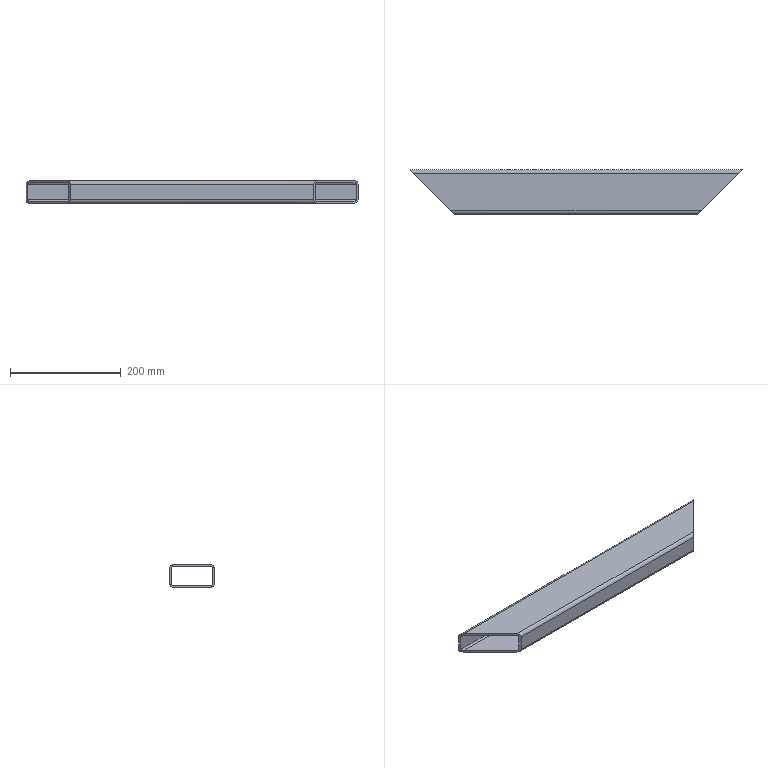Part | SolidWorks | features 3DProfileFeature 1, ICE 1, WeldMemberFeat 1, WeldmentFeature 1 | 1 solid | 18 faces | box 600 x 80 x 40 mm | volume 343628 mm3 | plane 10 | cylinder 8 | commonest cylinder face diameters 6 x4 12 x4
STEP:
#1=CARTESIAN_POINT('',(526.,-34.,-20.));
#2=VERTEX_POINT('',#1);
#3=CARTESIAN_POINT('',(594.,34.,-20.));
#4=VERTEX_POINT('',#3);
#5=CARTESIAN_POINT('',(280.,-280.,-20.));
#6=DIRECTION('',(0.7071,0.7071,0.));
#7=VECTOR('',#6,1000.);
#8=LINE('',#5,#7);
#9=EDGE_CURVE('',#2,#4,#8,.T.);
#10=ORIENTED_EDGE('',*,*,#9,.F.);
#11=CARTESIAN_POINT('',(74.,-34.,-20.));
#12=VERTEX_POINT('',#11);
#13=CARTESIAN_POINT('',(600.,-34.,-20.));
#14=DIRECTION('',(-1.,0.,0.));
#15=VECTOR('',#14,1000.);
#16=LINE('',#13,#15);
#17=EDGE_CURVE('',#2,#12,#16,.T.);
#18=ORIENTED_EDGE('',*,*,#17,.T.);
#19=CARTESIAN_POINT('',(6.,34.,-20.));
#20=VERTEX_POINT('',#19);
#21=CARTESIAN_POINT('',(20.,20.,-20.));
#22=DIRECTION('',(0.7071,-0.7071,0.));
#23=VECTOR('',#22,1000.);
#24=LINE('',#21,#23);
#25=EDGE_CURVE('',#20,#12,#24,.T.);
#26=ORIENTED_EDGE('',*,*,#25,.F.);
#27=CARTESIAN_POINT('',(600.,34.,-20.));
#28=DIRECTION('',(-1.,0.,0.));
#29=VECTOR('',#28,1000.);
#30=LINE('',#27,#29);
#31=EDGE_CURVE('',#4,#20,#30,.T.);
#32=ORIENTED_EDGE('',*,*,#31,.F.);
#33=EDGE_LOOP('',(#10,#18,#26,#32));
#34=FACE_OUTER_BOUND('',#33,.T.);
#35=CARTESIAN_POINT('',(600.,34.,-20.));
#36=DIRECTION('',(0.,0.,1.));
#37=DIRECTION('',(1.,0.,0.));
#38=AXIS2_PLACEMENT_3D('',#35,#36,#37);
#39=PLANE('',#38);
#40=ADVANCED_FACE('',(#34),#39,.F.);
#41=CARTESIAN_POINT('',(520.,-40.,-14.));
#42=VERTEX_POINT('',#41);
#43=CARTESIAN_POINT('',(520.,-40.,-14.));
#44=CARTESIAN_POINT('',(520.,-40.,-17.515));
#45=CARTESIAN_POINT('',(522.485,-37.515,-20.));
#46=CARTESIAN_POINT('',(526.,-34.,-20.));
#47=(BOUNDED_CURVE()B_SPLINE_CURVE(3,(#43,#44,#45,#46),.UNSPECIFIED.,.F.,.F.)B_SPLINE_CURVE_WITH_KNOTS((4,4),(0.,1.571),.UNSPECIFIED.)CURVE()GEOMETRIC_REPRESENTATION_ITEM()RATIONAL_B_SPLINE_CURVE((1.,0.8047,0.8047,1.))REPRESENTATION_ITEM(''));
#48=EDGE_CURVE('',#42,#2,#47,.T.);
#49=ORIENTED_EDGE('',*,*,#48,.F.);
#50=CARTESIAN_POINT('',(80.,-40.,-14.));
#51=VERTEX_POINT('',#50);
#52=CARTESIAN_POINT('',(600.,-40.,-14.));
#53=DIRECTION('',(-1.,0.,0.));
#54=VECTOR('',#53,1000.);
#55=LINE('',#52,#54);
#56=EDGE_CURVE('',#42,#51,#55,.T.);
#57=ORIENTED_EDGE('',*,*,#56,.T.);
#58=CARTESIAN_POINT('',(74.,-34.,-20.));
#59=CARTESIAN_POINT('',(77.515,-37.515,-20.));
#60=CARTESIAN_POINT('',(80.,-40.,-17.515));
#61=CARTESIAN_POINT('',(80.,-40.,-14.));
#62=(BOUNDED_CURVE()B_SPLINE_CURVE(3,(#58,#59,#60,#61),.UNSPECIFIED.,.F.,.F.)B_SPLINE_CURVE_WITH_KNOTS((4,4),(1.571,3.142),.UNSPECIFIED.)CURVE()GEOMETRIC_REPRESENTATION_ITEM()RATIONAL_B_SPLINE_CURVE((1.,0.8047,0.8047,1.))REPRESENTATION_ITEM(''));
#63=EDGE_CURVE('',#12,#51,#62,.T.);
#64=ORIENTED_EDGE('',*,*,#63,.F.);
#65=ORIENTED_EDGE('',*,*,#17,.F.);
#66=EDGE_LOOP('',(#49,#57,#64,#65));
#67=FACE_OUTER_BOUND('',#66,.T.);
#68=CARTESIAN_POINT('',(600.,-34.,-14.));
#69=DIRECTION('',(-1.,0.,0.));
#70=DIRECTION('',(0.,0.,1.));
#71=AXIS2_PLACEMENT_3D('',#68,#69,#70);
#72=CYLINDRICAL_SURFACE('',#71,6.);
#73=ADVANCED_FACE('',(#67),#72,.T.);
#74=CARTESIAN_POINT('',(520.,-40.,14.));
#75=VERTEX_POINT('',#74);
#76=CARTESIAN_POINT('',(520.,-40.,-20.));
#77=DIRECTION('',(0.,0.,1.));
#78=VECTOR('',#77,1000.);
#79=LINE('',#76,#78);
#80=EDGE_CURVE('',#42,#75,#79,.T.);
#81=ORIENTED_EDGE('',*,*,#80,.T.);
#82=CARTESIAN_POINT('',(80.,-40.,14.));
#83=VERTEX_POINT('',#82);
#84=CARTESIAN_POINT('',(600.,-40.,14.));
#85=DIRECTION('',(-1.,0.,0.));
#86=VECTOR('',#85,1000.);
#87=LINE('',#84,#86);
#88=EDGE_CURVE('',#75,#83,#87,.T.);
#89=ORIENTED_EDGE('',*,*,#88,.T.);
#90=CARTESIAN_POINT('',(80.,-40.,-20.));
#91=DIRECTION('',(0.,0.,1.));
#92=VECTOR('',#91,1000.);
#93=LINE('',#90,#92);
#94=EDGE_CURVE('',#51,#83,#93,.T.);
#95=ORIENTED_EDGE('',*,*,#94,.F.);
#96=ORIENTED_EDGE('',*,*,#56,.F.);
#97=EDGE_LOOP('',(#81,#89,#95,#96));
#98=FACE_OUTER_BOUND('',#97,.T.);
#99=CARTESIAN_POINT('',(600.,-40.,14.));
#100=DIRECTION('',(0.,1.,0.));
#101=DIRECTION('',(0.,0.,1.));
#102=AXIS2_PLACEMENT_3D('',#99,#100,#101);
#103=PLANE('',#102);
#104=ADVANCED_FACE('',(#98),#103,.F.);
#105=CARTESIAN_POINT('',(526.,-34.,20.));
#106=VERTEX_POINT('',#105);
#107=CARTESIAN_POINT('',(526.,-34.,20.));
#108=CARTESIAN_POINT('',(522.485,-37.515,20.));
#109=CARTESIAN_POINT('',(520.,-40.,17.515));
#110=CARTESIAN_POINT('',(520.,-40.,14.));
#111=(BOUNDED_CURVE()B_SPLINE_CURVE(3,(#107,#108,#109,#110),.UNSPECIFIED.,.F.,.F.)B_SPLINE_CURVE_WITH_KNOTS((4,4),(4.712,6.283),.UNSPECIFIED.)CURVE()GEOMETRIC_REPRESENTATION_ITEM()RATIONAL_B_SPLINE_CURVE((1.,0.8047,0.8047,1.))REPRESENTATION_ITEM(''));
#112=EDGE_CURVE('',#106,#75,#111,.T.);
#113=ORIENTED_EDGE('',*,*,#112,.F.);
#114=CARTESIAN_POINT('',(74.,-34.,20.));
#115=VERTEX_POINT('',#114);
#116=CARTESIAN_POINT('',(600.,-34.,20.));
#117=DIRECTION('',(-1.,0.,0.));
#118=VECTOR('',#117,1000.);
#119=LINE('',#116,#118);
#120=EDGE_CURVE('',#106,#115,#119,.T.);
#121=ORIENTED_EDGE('',*,*,#120,.T.);
#122=CARTESIAN_POINT('',(80.,-40.,14.));
#123=CARTESIAN_POINT('',(80.,-40.,17.515));
#124=CARTESIAN_POINT('',(77.515,-37.515,20.));
#125=CARTESIAN_POINT('',(74.,-34.,20.));
#126=(BOUNDED_CURVE()B_SPLINE_CURVE(3,(#122,#123,#124,#125),.UNSPECIFIED.,.F.,.F.)B_SPLINE_CURVE_WITH_KNOTS((4,4),(3.142,4.712),.UNSPECIFIED.)CURVE()GEOMETRIC_REPRESENTATION_ITEM()RATIONAL_B_SPLINE_CURVE((1.,0.8047,0.8047,1.))REPRESENTATION_ITEM(''));
#127=EDGE_CURVE('',#83,#115,#126,.T.);
#128=ORIENTED_EDGE('',*,*,#127,.F.);
#129=ORIENTED_EDGE('',*,*,#88,.F.);
#130=EDGE_LOOP('',(#113,#121,#128,#129));
#131=FACE_OUTER_BOUND('',#130,.T.);
#132=CARTESIAN_POINT('',(600.,-34.,14.));
#133=DIRECTION('',(-1.,0.,0.));
#134=DIRECTION('',(0.,0.,1.));
#135=AXIS2_PLACEMENT_3D('',#132,#133,#134);
#136=CYLINDRICAL_SURFACE('',#135,6.);
#137=ADVANCED_FACE('',(#131),#136,.T.);
#138=CARTESIAN_POINT('',(594.,34.,20.));
#139=VERTEX_POINT('',#138);
#140=CARTESIAN_POINT('',(280.,-280.,20.));
#141=DIRECTION('',(0.7071,0.7071,0.));
#142=VECTOR('',#141,1000.);
#143=LINE('',#140,#142);
#144=EDGE_CURVE('',#106,#139,#143,.T.);
#145=ORIENTED_EDGE('',*,*,#144,.T.);
#146=CARTESIAN_POINT('',(6.,34.,20.));
#147=VERTEX_POINT('',#146);
#148=CARTESIAN_POINT('',(600.,34.,20.));
#149=DIRECTION('',(-1.,0.,0.));
#150=VECTOR('',#149,1000.);
#151=LINE('',#148,#150);
#152=EDGE_CURVE('',#139,#147,#151,.T.);
#153=ORIENTED_EDGE('',*,*,#152,.T.);
#154=CARTESIAN_POINT('',(20.,20.,20.));
#155=DIRECTION('',(0.7071,-0.7071,0.));
#156=VECTOR('',#155,1000.);
#157=LINE('',#154,#156);
#158=EDGE_CURVE('',#147,#115,#157,.T.);
#159=ORIENTED_EDGE('',*,*,#158,.T.);
#160=ORIENTED_EDGE('',*,*,#120,.F.);
#161=EDGE_LOOP('',(#145,#153,#159,#160));
#162=FACE_OUTER_BOUND('',#161,.T.);
#163=CARTESIAN_POINT('',(600.,-34.,20.));
#164=DIRECTION('',(0.,0.,-1.));
#165=DIRECTION('',(-1.,0.,0.));
#166=AXIS2_PLACEMENT_3D('',#163,#164,#165);
#167=PLANE('',#166);
#168=ADVANCED_FACE('',(#162),#167,.F.);
#169=CARTESIAN_POINT('',(0.,40.,-14.));
#170=VERTEX_POINT('',#169);
#171=CARTESIAN_POINT('',(0.,40.,14.));
#172=VERTEX_POINT('',#171);
#173=CARTESIAN_POINT('',(0.,40.,-14.));
#174=DIRECTION('',(0.,0.,1.));
#175=VECTOR('',#174,1000.);
#176=LINE('',#173,#175);
#177=EDGE_CURVE('',#170,#172,#176,.T.);
#178=ORIENTED_EDGE('',*,*,#177,.T.);
#179=CARTESIAN_POINT('',(600.,40.,14.));
#180=VERTEX_POINT('',#179);
#181=CARTESIAN_POINT('',(600.,40.,14.));
#182=DIRECTION('',(-1.,0.,0.));
#183=VECTOR('',#182,1000.);
#184=LINE('',#181,#183);
#185=EDGE_CURVE('',#180,#172,#184,.T.);
#186=ORIENTED_EDGE('',*,*,#185,.F.);
#187=CARTESIAN_POINT('',(600.,40.,-14.));
#188=VERTEX_POINT('',#187);
#189=CARTESIAN_POINT('',(600.,40.,-14.));
#190=DIRECTION('',(0.,0.,1.));
#191=VECTOR('',#190,1000.);
#192=LINE('',#189,#191);
#193=EDGE_CURVE('',#188,#180,#192,.T.);
#194=ORIENTED_EDGE('',*,*,#193,.F.);
#195=CARTESIAN_POINT('',(600.,40.,-14.));
#196=DIRECTION('',(-1.,0.,0.));
#197=VECTOR('',#196,1000.);
#198=LINE('',#195,#197);
#199=EDGE_CURVE('',#188,#170,#198,.T.);
#200=ORIENTED_EDGE('',*,*,#199,.T.);
#201=EDGE_LOOP('',(#178,#186,#194,#200));
#202=FACE_OUTER_BOUND('',#201,.T.);
#203=CARTESIAN_POINT('',(600.,40.,-14.));
#204=DIRECTION('',(0.,-1.,0.));
#205=DIRECTION('',(0.,0.,-1.));
#206=AXIS2_PLACEMENT_3D('',#203,#204,#205);
#207=PLANE('',#206);
#208=ADVANCED_FACE('',(#202),#207,.F.);
#209=CARTESIAN_POINT('',(600.,40.,14.));
#210=CARTESIAN_POINT('',(600.,40.,17.515));
#211=CARTESIAN_POINT('',(597.515,37.515,20.));
#212=CARTESIAN_POINT('',(594.,34.,20.));
#213=(BOUNDED_CURVE()B_SPLINE_CURVE(3,(#209,#210,#211,#212),.UNSPECIFIED.,.F.,.F.)B_SPLINE_CURVE_WITH_KNOTS((4,4),(3.142,4.712),.UNSPECIFIED.)CURVE()GEOMETRIC_REPRESENTATION_ITEM()RATIONAL_B_SPLINE_CURVE((1.,0.8047,0.8047,1.))REPRESENTATION_ITEM(''));
#214=EDGE_CURVE('',#180,#139,#213,.T.);
#215=ORIENTED_EDGE('',*,*,#214,.F.);
#216=ORIENTED_EDGE('',*,*,#185,.T.);
#217=CARTESIAN_POINT('',(6.,34.,20.));
#218=CARTESIAN_POINT('',(2.485,37.515,20.));
#219=CARTESIAN_POINT('',(0.,40.,17.515));
#220=CARTESIAN_POINT('',(0.,40.,14.));
#221=(BOUNDED_CURVE()B_SPLINE_CURVE(3,(#217,#218,#219,#220),.UNSPECIFIED.,.F.,.F.)B_SPLINE_CURVE_WITH_KNOTS((4,4),(4.712,6.283),.UNSPECIFIED.)CURVE()GEOMETRIC_REPRESENTATION_ITEM()RATIONAL_B_SPLINE_CURVE((1.,0.8047,0.8047,1.))REPRESENTATION_ITEM(''));
#222=EDGE_CURVE('',#147,#172,#221,.T.);
#223=ORIENTED_EDGE('',*,*,#222,.F.);
#224=ORIENTED_EDGE('',*,*,#152,.F.);
#225=EDGE_LOOP('',(#215,#216,#223,#224));
#226=FACE_OUTER_BOUND('',#225,.T.);
#227=CARTESIAN_POINT('',(600.,34.,14.));
#228=DIRECTION('',(-1.,0.,0.));
#229=DIRECTION('',(0.,0.,1.));
#230=AXIS2_PLACEMENT_3D('',#227,#228,#229);
#231=CYLINDRICAL_SURFACE('',#230,6.);
#232=ADVANCED_FACE('',(#226),#231,.T.);
#233=CARTESIAN_POINT('',(594.,34.,-20.));
#234=CARTESIAN_POINT('',(597.515,37.515,-20.));
#235=CARTESIAN_POINT('',(600.,40.,-17.515));
#236=CARTESIAN_POINT('',(600.,40.,-14.));
#237=(BOUNDED_CURVE()B_SPLINE_CURVE(3,(#233,#234,#235,#236),.UNSPECIFIED.,.F.,.F.)B_SPLINE_CURVE_WITH_KNOTS((4,4),(1.571,3.142),.UNSPECIFIED.)CURVE()GEOMETRIC_REPRESENTATION_ITEM()RATIONAL_B_SPLINE_CURVE((1.,0.8047,0.8047,1.))REPRESENTATION_ITEM(''));
#238=EDGE_CURVE('',#4,#188,#237,.T.);
#239=ORIENTED_EDGE('',*,*,#238,.F.);
#240=ORIENTED_EDGE('',*,*,#31,.T.);
#241=CARTESIAN_POINT('',(0.,40.,-14.));
#242=CARTESIAN_POINT('',(0.,40.,-17.515));
#243=CARTESIAN_POINT('',(2.485,37.515,-20.));
#244=CARTESIAN_POINT('',(6.,34.,-20.));
#245=(BOUNDED_CURVE()B_SPLINE_CURVE(3,(#241,#242,#243,#244),.UNSPECIFIED.,.F.,.F.)B_SPLINE_CURVE_WITH_KNOTS((4,4),(0.,1.571),.UNSPECIFIED.)CURVE()GEOMETRIC_REPRESENTATION_ITEM()RATIONAL_B_SPLINE_CURVE((1.,0.8047,0.8047,1.))REPRESENTATION_ITEM(''));
#246=EDGE_CURVE('',#170,#20,#245,.T.);
#247=ORIENTED_EDGE('',*,*,#246,.F.);
#248=ORIENTED_EDGE('',*,*,#199,.F.);
#249=EDGE_LOOP('',(#239,#240,#247,#248));
#250=FACE_OUTER_BOUND('',#249,.T.);
#251=CARTESIAN_POINT('',(600.,34.,-14.));
#252=DIRECTION('',(-1.,0.,0.));
#253=DIRECTION('',(0.,0.,1.));
#254=AXIS2_PLACEMENT_3D('',#251,#252,#253);
#255=CYLINDRICAL_SURFACE('',#254,6.);
#256=ADVANCED_FACE('',(#250),#255,.T.);
#257=CARTESIAN_POINT('',(74.,-34.,17.));
#258=VERTEX_POINT('',#257);
#259=CARTESIAN_POINT('',(6.,34.,17.));
#260=VERTEX_POINT('',#259);
#261=CARTESIAN_POINT('',(337.,-297.,17.));
#262=DIRECTION('',(-0.7071,0.7071,0.));
#263=VECTOR('',#262,1000.);
#264=LINE('',#261,#263);
#265=EDGE_CURVE('',#258,#260,#264,.T.);
#266=ORIENTED_EDGE('',*,*,#265,.F.);
#267=CARTESIAN_POINT('',(77.,-37.,14.));
#268=VERTEX_POINT('',#267);
#269=CARTESIAN_POINT('',(77.,-37.,14.));
#270=CARTESIAN_POINT('',(77.,-37.,15.757));
#271=CARTESIAN_POINT('',(75.757,-35.757,17.));
#272=CARTESIAN_POINT('',(74.,-34.,17.));
#273=(BOUNDED_CURVE()B_SPLINE_CURVE(3,(#269,#270,#271,#272),.UNSPECIFIED.,.F.,.T.)B_SPLINE_CURVE_WITH_KNOTS((4,4),(3.142,4.712),.UNSPECIFIED.)CURVE()GEOMETRIC_REPRESENTATION_ITEM()RATIONAL_B_SPLINE_CURVE((1.,0.8047,0.8047,1.))REPRESENTATION_ITEM(''));
#274=EDGE_CURVE('',#268,#258,#273,.T.);
#275=ORIENTED_EDGE('',*,*,#274,.F.);
#276=CARTESIAN_POINT('',(77.,-37.,-14.));
#277=VERTEX_POINT('',#276);
#278=CARTESIAN_POINT('',(77.,-37.,14.));
#279=DIRECTION('',(0.,0.,1.));
#280=VECTOR('',#279,1000.);
#281=LINE('',#278,#280);
#282=EDGE_CURVE('',#277,#268,#281,.T.);
#283=ORIENTED_EDGE('',*,*,#282,.F.);
#284=CARTESIAN_POINT('',(74.,-34.,-17.));
#285=VERTEX_POINT('',#284);
#286=CARTESIAN_POINT('',(74.,-34.,-17.));
#287=CARTESIAN_POINT('',(75.757,-35.757,-17.));
#288=CARTESIAN_POINT('',(77.,-37.,-15.757));
#289=CARTESIAN_POINT('',(77.,-37.,-14.));
#290=(BOUNDED_CURVE()B_SPLINE_CURVE(3,(#286,#287,#288,#289),.UNSPECIFIED.,.F.,.F.)B_SPLINE_CURVE_WITH_KNOTS((4,4),(1.571,3.142),.UNSPECIFIED.)CURVE()GEOMETRIC_REPRESENTATION_ITEM()RATIONAL_B_SPLINE_CURVE((1.,0.8047,0.8047,1.))REPRESENTATION_ITEM(''));
#291=EDGE_CURVE('',#285,#277,#290,.T.);
#292=ORIENTED_EDGE('',*,*,#291,.F.);
#293=CARTESIAN_POINT('',(6.,34.,-17.));
#294=VERTEX_POINT('',#293);
#295=CARTESIAN_POINT('',(303.,-263.,-17.));
#296=DIRECTION('',(0.7071,-0.7071,0.));
#297=VECTOR('',#296,1000.);
#298=LINE('',#295,#297);
#299=EDGE_CURVE('',#294,#285,#298,.T.);
#300=ORIENTED_EDGE('',*,*,#299,.F.);
#301=CARTESIAN_POINT('',(3.,37.,-14.));
#302=VERTEX_POINT('',#301);
#303=CARTESIAN_POINT('',(3.,37.,-14.));
#304=CARTESIAN_POINT('',(3.,37.,-15.757));
#305=CARTESIAN_POINT('',(4.243,35.757,-17.));
#306=CARTESIAN_POINT('',(6.,34.,-17.));
#307=(BOUNDED_CURVE()B_SPLINE_CURVE(3,(#303,#304,#305,#306),.UNSPECIFIED.,.F.,.F.)B_SPLINE_CURVE_WITH_KNOTS((4,4),(0.,1.571),.UNSPECIFIED.)CURVE()GEOMETRIC_REPRESENTATION_ITEM()RATIONAL_B_SPLINE_CURVE((1.,0.8047,0.8047,1.))REPRESENTATION_ITEM(''));
#308=EDGE_CURVE('',#302,#294,#307,.T.);
#309=ORIENTED_EDGE('',*,*,#308,.F.);
#310=CARTESIAN_POINT('',(3.,37.,14.));
#311=VERTEX_POINT('',#310);
#312=CARTESIAN_POINT('',(3.,37.,-14.));
#313=DIRECTION('',(0.,0.,-1.));
#314=VECTOR('',#313,1000.);
#315=LINE('',#312,#314);
#316=EDGE_CURVE('',#311,#302,#315,.T.);
#317=ORIENTED_EDGE('',*,*,#316,.F.);
#318=CARTESIAN_POINT('',(6.,34.,17.));
#319=CARTESIAN_POINT('',(4.243,35.757,17.));
#320=CARTESIAN_POINT('',(3.,37.,15.757));
#321=CARTESIAN_POINT('',(3.,37.,14.));
#322=(BOUNDED_CURVE()B_SPLINE_CURVE(3,(#318,#319,#320,#321),.UNSPECIFIED.,.F.,.F.)B_SPLINE_CURVE_WITH_KNOTS((4,4),(4.712,6.283),.UNSPECIFIED.)CURVE()GEOMETRIC_REPRESENTATION_ITEM()RATIONAL_B_SPLINE_CURVE((1.,0.8047,0.8047,1.))REPRESENTATION_ITEM(''));
#323=EDGE_CURVE('',#260,#311,#322,.T.);
#324=ORIENTED_EDGE('',*,*,#323,.F.);
#325=EDGE_LOOP('',(#266,#275,#283,#292,#300,#309,#317,#324));
#326=FACE_BOUND('',#325,.T.);
#327=ORIENTED_EDGE('',*,*,#246,.T.);
#328=ORIENTED_EDGE('',*,*,#25,.T.);
#329=ORIENTED_EDGE('',*,*,#63,.T.);
#330=ORIENTED_EDGE('',*,*,#94,.T.);
#331=ORIENTED_EDGE('',*,*,#127,.T.);
#332=ORIENTED_EDGE('',*,*,#158,.F.);
#333=ORIENTED_EDGE('',*,*,#222,.T.);
#334=ORIENTED_EDGE('',*,*,#177,.F.);
#335=EDGE_LOOP('',(#327,#328,#329,#330,#331,#332,#333,#334));
#336=FACE_OUTER_BOUND('',#335,.T.);
#337=CARTESIAN_POINT('',(20.,20.,-20.));
#338=DIRECTION('',(-0.7071,-0.7071,0.));
#339=DIRECTION('',(0.7071,-0.7071,0.));
#340=AXIS2_PLACEMENT_3D('',#337,#338,#339);
#341=PLANE('',#340);
#342=ADVANCED_FACE('',(#326,#336),#341,.T.);
#343=CARTESIAN_POINT('',(597.,37.,-14.));
#344=VERTEX_POINT('',#343);
#345=CARTESIAN_POINT('',(597.,37.,14.));
#346=VERTEX_POINT('',#345);
#347=CARTESIAN_POINT('',(597.,37.,-14.));
#348=DIRECTION('',(0.,0.,1.));
#349=VECTOR('',#348,1000.);
#350=LINE('',#347,#349);
#351=EDGE_CURVE('',#344,#346,#350,.T.);
#352=ORIENTED_EDGE('',*,*,#351,.F.);
#353=CARTESIAN_POINT('',(594.,34.,-17.));
#354=VERTEX_POINT('',#353);
#355=CARTESIAN_POINT('',(594.,34.,-17.));
#356=CARTESIAN_POINT('',(595.757,35.757,-17.));
#357=CARTESIAN_POINT('',(597.,37.,-15.757));
#358=CARTESIAN_POINT('',(597.,37.,-14.));
#359=(BOUNDED_CURVE()B_SPLINE_CURVE(3,(#355,#356,#357,#358),.UNSPECIFIED.,.F.,.F.)B_SPLINE_CURVE_WITH_KNOTS((4,4),(1.571,3.142),.UNSPECIFIED.)CURVE()GEOMETRIC_REPRESENTATION_ITEM()RATIONAL_B_SPLINE_CURVE((1.,0.8047,0.8047,1.))REPRESENTATION_ITEM(''));
#360=EDGE_CURVE('',#354,#344,#359,.T.);
#361=ORIENTED_EDGE('',*,*,#360,.F.);
#362=CARTESIAN_POINT('',(526.,-34.,-17.));
#363=VERTEX_POINT('',#362);
#364=CARTESIAN_POINT('',(597.,37.,-17.));
#365=DIRECTION('',(0.7071,0.7071,0.));
#366=VECTOR('',#365,1000.);
#367=LINE('',#364,#366);
#368=EDGE_CURVE('',#363,#354,#367,.T.);
#369=ORIENTED_EDGE('',*,*,#368,.F.);
#370=CARTESIAN_POINT('',(523.,-37.,-14.));
#371=VERTEX_POINT('',#370);
#372=CARTESIAN_POINT('',(523.,-37.,-14.));
#373=CARTESIAN_POINT('',(523.,-37.,-15.757));
#374=CARTESIAN_POINT('',(524.243,-35.757,-17.));
#375=CARTESIAN_POINT('',(526.,-34.,-17.));
#376=(BOUNDED_CURVE()B_SPLINE_CURVE(3,(#372,#373,#374,#375),.UNSPECIFIED.,.F.,.F.)B_SPLINE_CURVE_WITH_KNOTS((4,4),(0.,1.571),.UNSPECIFIED.)CURVE()GEOMETRIC_REPRESENTATION_ITEM()RATIONAL_B_SPLINE_CURVE((1.,0.8047,0.8047,1.))REPRESENTATION_ITEM(''));
#377=EDGE_CURVE('',#371,#363,#376,.T.);
#378=ORIENTED_EDGE('',*,*,#377,.F.);
#379=CARTESIAN_POINT('',(523.,-37.,14.));
#380=VERTEX_POINT('',#379);
#381=CARTESIAN_POINT('',(523.,-37.,14.));
#382=DIRECTION('',(0.,0.,-1.));
#383=VECTOR('',#382,1000.);
#384=LINE('',#381,#383);
#385=EDGE_CURVE('',#380,#371,#384,.T.);
#386=ORIENTED_EDGE('',*,*,#385,.F.);
#387=CARTESIAN_POINT('',(526.,-34.,17.));
#388=VERTEX_POINT('',#387);
#389=CARTESIAN_POINT('',(526.,-34.,17.));
#390=CARTESIAN_POINT('',(524.243,-35.757,17.));
#391=CARTESIAN_POINT('',(523.,-37.,15.757));
#392=CARTESIAN_POINT('',(523.,-37.,14.));
#393=(BOUNDED_CURVE()B_SPLINE_CURVE(3,(#389,#390,#391,#392),.UNSPECIFIED.,.F.,.F.)B_SPLINE_CURVE_WITH_KNOTS((4,4),(4.712,6.283),.UNSPECIFIED.)CURVE()GEOMETRIC_REPRESENTATION_ITEM()RATIONAL_B_SPLINE_CURVE((1.,0.8047,0.8047,1.))REPRESENTATION_ITEM(''));
#394=EDGE_CURVE('',#388,#380,#393,.T.);
#395=ORIENTED_EDGE('',*,*,#394,.F.);
#396=CARTESIAN_POINT('',(594.,34.,17.));
#397=VERTEX_POINT('',#396);
#398=CARTESIAN_POINT('',(563.,3.,17.));
#399=DIRECTION('',(-0.7071,-0.7071,0.));
#400=VECTOR('',#399,1000.);
#401=LINE('',#398,#400);
#402=EDGE_CURVE('',#397,#388,#401,.T.);
#403=ORIENTED_EDGE('',*,*,#402,.F.);
#404=CARTESIAN_POINT('',(597.,37.,14.));
#405=CARTESIAN_POINT('',(597.,37.,15.757));
#406=CARTESIAN_POINT('',(595.757,35.757,17.));
#407=CARTESIAN_POINT('',(594.,34.,17.));
#408=(BOUNDED_CURVE()B_SPLINE_CURVE(3,(#404,#405,#406,#407),.UNSPECIFIED.,.F.,.F.)B_SPLINE_CURVE_WITH_KNOTS((4,4),(3.142,4.712),.UNSPECIFIED.)CURVE()GEOMETRIC_REPRESENTATION_ITEM()RATIONAL_B_SPLINE_CURVE((1.,0.8047,0.8047,1.))REPRESENTATION_ITEM(''));
#409=EDGE_CURVE('',#346,#397,#408,.T.);
#410=ORIENTED_EDGE('',*,*,#409,.F.);
#411=EDGE_LOOP('',(#352,#361,#369,#378,#386,#395,#403,#410));
#412=FACE_BOUND('',#411,.T.);
#413=ORIENTED_EDGE('',*,*,#238,.T.);
#414=ORIENTED_EDGE('',*,*,#193,.T.);
#415=ORIENTED_EDGE('',*,*,#214,.T.);
#416=ORIENTED_EDGE('',*,*,#144,.F.);
#417=ORIENTED_EDGE('',*,*,#112,.T.);
#418=ORIENTED_EDGE('',*,*,#80,.F.);
#419=ORIENTED_EDGE('',*,*,#48,.T.);
#420=ORIENTED_EDGE('',*,*,#9,.T.);
#421=EDGE_LOOP('',(#413,#414,#415,#416,#417,#418,#419,#420));
#422=FACE_OUTER_BOUND('',#421,.T.);
#423=CARTESIAN_POINT('',(280.,-280.,-20.));
#424=DIRECTION('',(0.7071,-0.7071,0.));
#425=DIRECTION('',(0.7071,0.7071,0.));
#426=AXIS2_PLACEMENT_3D('',#423,#424,#425);
#427=PLANE('',#426);
#428=ADVANCED_FACE('',(#412,#422),#427,.T.);
#429=CARTESIAN_POINT('',(600.,37.,14.));
#430=DIRECTION('',(-1.,0.,0.));
#431=VECTOR('',#430,1000.);
#432=LINE('',#429,#431);
#433=EDGE_CURVE('',#346,#311,#432,.T.);
#434=ORIENTED_EDGE('',*,*,#433,.F.);
#435=ORIENTED_EDGE('',*,*,#409,.T.);
#436=CARTESIAN_POINT('',(600.,34.,17.));
#437=DIRECTION('',(-1.,0.,0.));
#438=VECTOR('',#437,1000.);
#439=LINE('',#436,#438);
#440=EDGE_CURVE('',#397,#260,#439,.T.);
#441=ORIENTED_EDGE('',*,*,#440,.T.);
#442=ORIENTED_EDGE('',*,*,#323,.T.);
#443=EDGE_LOOP('',(#434,#435,#441,#442));
#444=FACE_OUTER_BOUND('',#443,.T.);
#445=CARTESIAN_POINT('',(600.,34.,14.));
#446=DIRECTION('',(-1.,0.,0.));
#447=DIRECTION('',(0.,0.,1.));
#448=AXIS2_PLACEMENT_3D('',#445,#446,#447);
#449=CYLINDRICAL_SURFACE('',#448,3.);
#450=ADVANCED_FACE('',(#444),#449,.F.);
#451=CARTESIAN_POINT('',(600.,37.,-14.));
#452=DIRECTION('',(-1.,0.,0.));
#453=VECTOR('',#452,1000.);
#454=LINE('',#451,#453);
#455=EDGE_CURVE('',#344,#302,#454,.T.);
#456=ORIENTED_EDGE('',*,*,#455,.F.);
#457=ORIENTED_EDGE('',*,*,#351,.T.);
#458=ORIENTED_EDGE('',*,*,#433,.T.);
#459=ORIENTED_EDGE('',*,*,#316,.T.);
#460=EDGE_LOOP('',(#456,#457,#458,#459));
#461=FACE_OUTER_BOUND('',#460,.T.);
#462=CARTESIAN_POINT('',(600.,37.,-14.));
#463=DIRECTION('',(0.,-1.,0.));
#464=DIRECTION('',(0.,0.,-1.));
#465=AXIS2_PLACEMENT_3D('',#462,#463,#464);
#466=PLANE('',#465);
#467=ADVANCED_FACE('',(#461),#466,.T.);
#468=CARTESIAN_POINT('',(600.,34.,-17.));
#469=DIRECTION('',(-1.,0.,0.));
#470=VECTOR('',#469,1000.);
#471=LINE('',#468,#470);
#472=EDGE_CURVE('',#354,#294,#471,.T.);
#473=ORIENTED_EDGE('',*,*,#472,.F.);
#474=ORIENTED_EDGE('',*,*,#360,.T.);
#475=ORIENTED_EDGE('',*,*,#455,.T.);
#476=ORIENTED_EDGE('',*,*,#308,.T.);
#477=EDGE_LOOP('',(#473,#474,#475,#476));
#478=FACE_OUTER_BOUND('',#477,.T.);
#479=CARTESIAN_POINT('',(600.,34.,-14.));
#480=DIRECTION('',(-1.,0.,0.));
#481=DIRECTION('',(0.,0.,1.));
#482=AXIS2_PLACEMENT_3D('',#479,#480,#481);
#483=CYLINDRICAL_SURFACE('',#482,3.);
#484=ADVANCED_FACE('',(#478),#483,.F.);
#485=CARTESIAN_POINT('',(600.,-34.,-17.));
#486=DIRECTION('',(-1.,0.,0.));
#487=VECTOR('',#486,1000.);
#488=LINE('',#485,#487);
#489=EDGE_CURVE('',#363,#285,#488,.T.);
#490=ORIENTED_EDGE('',*,*,#489,.F.);
#491=ORIENTED_EDGE('',*,*,#368,.T.);
#492=ORIENTED_EDGE('',*,*,#472,.T.);
#493=ORIENTED_EDGE('',*,*,#299,.T.);
#494=EDGE_LOOP('',(#490,#491,#492,#493));
#495=FACE_OUTER_BOUND('',#494,.T.);
#496=CARTESIAN_POINT('',(600.,34.,-17.));
#497=DIRECTION('',(0.,0.,1.));
#498=DIRECTION('',(1.,0.,0.));
#499=AXIS2_PLACEMENT_3D('',#496,#497,#498);
#500=PLANE('',#499);
#501=ADVANCED_FACE('',(#495),#500,.T.);
#502=CARTESIAN_POINT('',(600.,-37.,-14.));
#503=DIRECTION('',(-1.,0.,0.));
#504=VECTOR('',#503,1000.);
#505=LINE('',#502,#504);
#506=EDGE_CURVE('',#371,#277,#505,.T.);
#507=ORIENTED_EDGE('',*,*,#506,.F.);
#508=ORIENTED_EDGE('',*,*,#377,.T.);
#509=ORIENTED_EDGE('',*,*,#489,.T.);
#510=ORIENTED_EDGE('',*,*,#291,.T.);
#511=EDGE_LOOP('',(#507,#508,#509,#510));
#512=FACE_OUTER_BOUND('',#511,.T.);
#513=CARTESIAN_POINT('',(600.,-34.,-14.));
#514=DIRECTION('',(-1.,0.,0.));
#515=DIRECTION('',(0.,0.,1.));
#516=AXIS2_PLACEMENT_3D('',#513,#514,#515);
#517=CYLINDRICAL_SURFACE('',#516,3.);
#518=ADVANCED_FACE('',(#512),#517,.F.);
#519=CARTESIAN_POINT('',(600.,-37.,14.));
#520=DIRECTION('',(-1.,0.,0.));
#521=VECTOR('',#520,1000.);
#522=LINE('',#519,#521);
#523=EDGE_CURVE('',#380,#268,#522,.T.);
#524=ORIENTED_EDGE('',*,*,#523,.F.);
#525=ORIENTED_EDGE('',*,*,#385,.T.);
#526=ORIENTED_EDGE('',*,*,#506,.T.);
#527=ORIENTED_EDGE('',*,*,#282,.T.);
#528=EDGE_LOOP('',(#524,#525,#526,#527));
#529=FACE_OUTER_BOUND('',#528,.T.);
#530=CARTESIAN_POINT('',(600.,-37.,14.));
#531=DIRECTION('',(0.,1.,0.));
#532=DIRECTION('',(0.,0.,1.));
#533=AXIS2_PLACEMENT_3D('',#530,#531,#532);
#534=PLANE('',#533);
#535=ADVANCED_FACE('',(#529),#534,.T.);
#536=CARTESIAN_POINT('',(600.,-34.,17.));
#537=DIRECTION('',(-1.,0.,0.));
#538=VECTOR('',#537,1000.);
#539=LINE('',#536,#538);
#540=EDGE_CURVE('',#388,#258,#539,.T.);
#541=ORIENTED_EDGE('',*,*,#540,.F.);
#542=ORIENTED_EDGE('',*,*,#394,.T.);
#543=ORIENTED_EDGE('',*,*,#523,.T.);
#544=ORIENTED_EDGE('',*,*,#274,.T.);
#545=EDGE_LOOP('',(#541,#542,#543,#544));
#546=FACE_OUTER_BOUND('',#545,.T.);
#547=CARTESIAN_POINT('',(600.,-34.,14.));
#548=DIRECTION('',(-1.,0.,0.));
#549=DIRECTION('',(0.,0.,1.));
#550=AXIS2_PLACEMENT_3D('',#547,#548,#549);
#551=CYLINDRICAL_SURFACE('',#550,3.);
#552=ADVANCED_FACE('',(#546),#551,.F.);
#553=ORIENTED_EDGE('',*,*,#440,.F.);
#554=ORIENTED_EDGE('',*,*,#402,.T.);
#555=ORIENTED_EDGE('',*,*,#540,.T.);
#556=ORIENTED_EDGE('',*,*,#265,.T.);
#557=EDGE_LOOP('',(#553,#554,#555,#556));
#558=FACE_OUTER_BOUND('',#557,.T.);
#559=CARTESIAN_POINT('',(600.,-34.,17.));
#560=DIRECTION('',(0.,0.,-1.));
#561=DIRECTION('',(-1.,0.,0.));
#562=AXIS2_PLACEMENT_3D('',#559,#560,#561);
#563=PLANE('',#562);
#564=ADVANCED_FACE('',(#558),#563,.T.);
#565=CLOSED_SHELL('',(#40,#73,#104,#137,#168,#208,#232,#256,#342,#428,#450,#467,#484,#501,#518,#535,#552,#564));
#566=MANIFOLD_SOLID_BREP('',#565);
#567=CARTESIAN_POINT('',(0.,0.,0.));
#568=DIRECTION('',(0.,0.,1.));
#569=DIRECTION('',(1.,0.,0.));
#570=AXIS2_PLACEMENT_3D('',#567,#568,#569);
#571=(LENGTH_UNIT()NAMED_UNIT(*)SI_UNIT(.MILLI.,.METRE.));
#572=UNCERTAINTY_MEASURE_WITH_UNIT(LENGTH_MEASURE(0.00001),#571,'','');
#573=(NAMED_UNIT(*)PLANE_ANGLE_UNIT()SI_UNIT($,.RADIAN.));
#574=(NAMED_UNIT(*)SI_UNIT($,.STERADIAN.)SOLID_ANGLE_UNIT());
#575=(GEOMETRIC_REPRESENTATION_CONTEXT(3)GLOBAL_UNCERTAINTY_ASSIGNED_CONTEXT((#572))GLOBAL_UNIT_ASSIGNED_CONTEXT((#571,#573,#574))REPRESENTATION_CONTEXT('',''));
#576=ADVANCED_BREP_SHAPE_REPRESENTATION('',(#566,#570),#575);